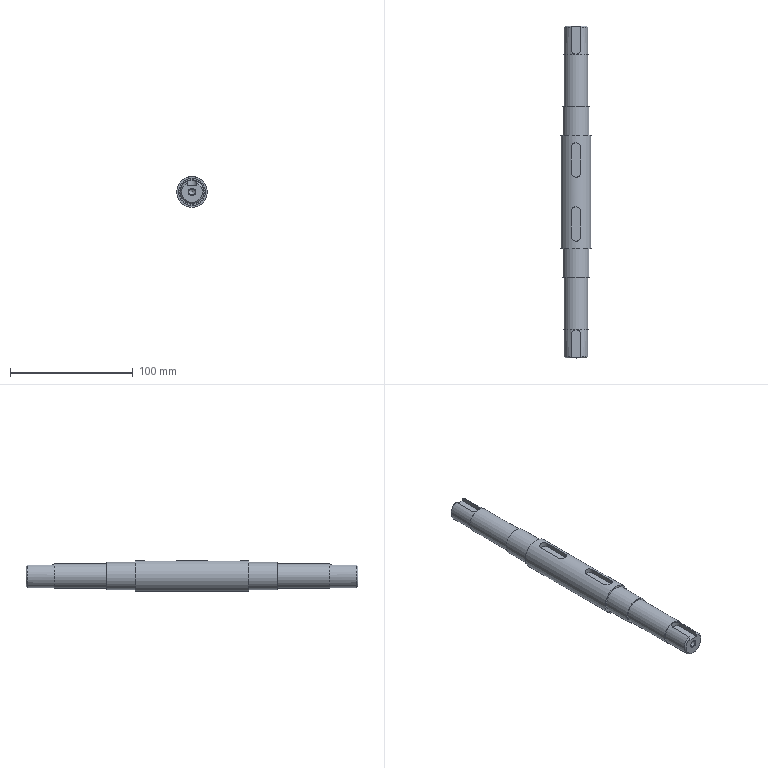Part | STEP file | 冲床-300配套压波_id430_x_t | 1 solid | 41 faces | box 25 x 270 x 25 mm | volume 98996 mm3 | plane 20 | cylinder 15 | cone 6 | commonest cylinder face diameters 8 x6 5 x2 19 x2 20 x2 22 x2 25 x1
STEP:
#1=CARTESIAN_POINT('',(1392.,115.,77.583));
#2=VERTEX_POINT('',#1);
#3=CARTESIAN_POINT('',(1392.,115.,80.083));
#4=DIRECTION('',(0.,1.,0.));
#5=DIRECTION('',(0.,0.,-1.));
#6=AXIS2_PLACEMENT_3D('',#3,#4,#5);
#7=CIRCLE('',#6,2.5);
#8=EDGE_CURVE('',#2,#2,#7,.T.);
#9=ORIENTED_EDGE('',*,*,#8,.T.);
#10=EDGE_LOOP('',(#9));
#11=FACE_BOUND('',#10,.T.);
#12=CARTESIAN_POINT('',(1392.,113.498,80.083));
#13=VERTEX_POINT('',#12);
#14=VERTEX_LOOP('',#13);
#15=FACE_BOUND('',#14,.T.);
#16=CARTESIAN_POINT('',(1392.,115.,80.083));
#17=DIRECTION('',(0.,1.,0.));
#18=DIRECTION('',(0.,0.,1.));
#19=AXIS2_PLACEMENT_3D('',#16,#17,#18);
#20=CONICAL_SURFACE('',#19,2.5,59.);
#21=ADVANCED_FACE('',(#11,#15),#20,.F.);
#22=CARTESIAN_POINT('',(1392.,134.5,77.583));
#23=VERTEX_POINT('',#22);
#24=CARTESIAN_POINT('',(1392.,134.5,80.083));
#25=DIRECTION('',(0.,1.,0.));
#26=DIRECTION('',(0.,0.,-1.));
#27=AXIS2_PLACEMENT_3D('',#24,#25,#26);
#28=CIRCLE('',#27,2.5);
#29=EDGE_CURVE('',#23,#23,#28,.T.);
#30=ORIENTED_EDGE('',*,*,#29,.T.);
#31=EDGE_LOOP('',(#30));
#32=FACE_BOUND('',#31,.T.);
#33=ORIENTED_EDGE('',*,*,#8,.F.);
#34=EDGE_LOOP('',(#33));
#35=FACE_BOUND('',#34,.T.);
#36=CARTESIAN_POINT('',(1392.,135.,80.083));
#37=DIRECTION('',(0.,-1.,0.));
#38=DIRECTION('',(0.,0.,-1.));
#39=AXIS2_PLACEMENT_3D('',#36,#37,#38);
#40=CYLINDRICAL_SURFACE('',#39,2.5);
#41=ADVANCED_FACE('',(#32,#35),#40,.F.);
#42=ORIENTED_EDGE('',*,*,#29,.F.);
#43=EDGE_LOOP('',(#42));
#44=FACE_BOUND('',#43,.T.);
#45=CARTESIAN_POINT('',(1392.,135.,77.083));
#46=VERTEX_POINT('',#45);
#47=CARTESIAN_POINT('',(1392.,135.,80.083));
#48=DIRECTION('',(0.,-1.,0.));
#49=DIRECTION('',(0.,0.,-1.));
#50=AXIS2_PLACEMENT_3D('',#47,#48,#49);
#51=CIRCLE('',#50,3.);
#52=EDGE_CURVE('',#46,#46,#51,.T.);
#53=ORIENTED_EDGE('',*,*,#52,.F.);
#54=EDGE_LOOP('',(#53));
#55=FACE_BOUND('',#54,.T.);
#56=CARTESIAN_POINT('',(1392.,135.,80.083));
#57=DIRECTION('',(0.,1.,0.));
#58=DIRECTION('',(0.,0.,1.));
#59=AXIS2_PLACEMENT_3D('',#56,#57,#58);
#60=CONICAL_SURFACE('',#59,3.,45.);
#61=ADVANCED_FACE('',(#44,#55),#60,.F.);
#62=CARTESIAN_POINT('',(1396.,116.,85.583));
#63=VERTEX_POINT('',#62);
#64=CARTESIAN_POINT('',(1396.,135.,85.583));
#65=VERTEX_POINT('',#64);
#66=CARTESIAN_POINT('',(1396.,114.5,85.583));
#67=DIRECTION('',(0.,1.,0.));
#68=VECTOR('',#67,1.);
#69=LINE('',#66,#68);
#70=EDGE_CURVE('',#63,#65,#69,.T.);
#71=ORIENTED_EDGE('',*,*,#70,.T.);
#72=CARTESIAN_POINT('',(1388.,135.,85.583));
#73=VERTEX_POINT('',#72);
#74=CARTESIAN_POINT('',(1392.,135.,85.583));
#75=DIRECTION('',(1.,0.,0.));
#76=VECTOR('',#75,1.);
#77=LINE('',#74,#76);
#78=EDGE_CURVE('',#73,#65,#77,.T.);
#79=ORIENTED_EDGE('',*,*,#78,.F.);
#80=CARTESIAN_POINT('',(1388.,116.,85.583));
#81=VERTEX_POINT('',#80);
#82=CARTESIAN_POINT('',(1388.,139.499,85.583));
#83=DIRECTION('',(0.,-1.,0.));
#84=VECTOR('',#83,1.);
#85=LINE('',#82,#84);
#86=EDGE_CURVE('',#73,#81,#85,.T.);
#87=ORIENTED_EDGE('',*,*,#86,.T.);
#88=CARTESIAN_POINT('',(1392.,116.,85.583));
#89=DIRECTION('',(0.,0.,1.));
#90=DIRECTION('',(1.,0.,0.));
#91=AXIS2_PLACEMENT_3D('',#88,#89,#90);
#92=CIRCLE('',#91,4.);
#93=EDGE_CURVE('',#81,#63,#92,.T.);
#94=ORIENTED_EDGE('',*,*,#93,.T.);
#95=EDGE_LOOP('',(#71,#79,#87,#94));
#96=FACE_OUTER_BOUND('',#95,.T.);
#97=CARTESIAN_POINT('',(1392.,114.5,85.583));
#98=DIRECTION('',(0.,0.,-1.));
#99=DIRECTION('',(-1.,0.,0.));
#100=AXIS2_PLACEMENT_3D('',#97,#98,#99);
#101=PLANE('',#100);
#102=ADVANCED_FACE('',(#96),#101,.F.);
#103=ORIENTED_EDGE('',*,*,#52,.T.);
#104=EDGE_LOOP('',(#103));
#105=FACE_BOUND('',#104,.T.);
#106=CARTESIAN_POINT('',(1396.,135.,87.583));
#107=VERTEX_POINT('',#106);
#108=CARTESIAN_POINT('',(1396.,135.,80.083));
#109=DIRECTION('',(0.,0.,-1.));
#110=VECTOR('',#109,1.);
#111=LINE('',#108,#110);
#112=EDGE_CURVE('',#107,#65,#111,.T.);
#113=ORIENTED_EDGE('',*,*,#112,.F.);
#114=CARTESIAN_POINT('',(1388.,135.,87.583));
#115=VERTEX_POINT('',#114);
#116=CARTESIAN_POINT('',(1392.,135.,80.083));
#117=DIRECTION('',(0.,1.,0.));
#118=DIRECTION('',(0.,0.,-1.));
#119=AXIS2_PLACEMENT_3D('',#116,#117,#118);
#120=CIRCLE('',#119,8.5);
#121=EDGE_CURVE('',#107,#115,#120,.T.);
#122=ORIENTED_EDGE('',*,*,#121,.T.);
#123=CARTESIAN_POINT('',(1388.,135.,80.083));
#124=DIRECTION('',(0.,0.,1.));
#125=VECTOR('',#124,1.);
#126=LINE('',#123,#125);
#127=EDGE_CURVE('',#73,#115,#126,.T.);
#128=ORIENTED_EDGE('',*,*,#127,.F.);
#129=ORIENTED_EDGE('',*,*,#78,.T.);
#130=EDGE_LOOP('',(#113,#122,#128,#129));
#131=FACE_BOUND('',#130,.T.);
#132=CARTESIAN_POINT('',(1392.,135.,80.083));
#133=DIRECTION('',(0.,-1.,0.));
#134=DIRECTION('',(-1.,0.,0.));
#135=AXIS2_PLACEMENT_3D('',#132,#133,#134);
#136=PLANE('',#135);
#137=ADVANCED_FACE('',(#105,#131),#136,.F.);
#138=CARTESIAN_POINT('',(1388.,116.,88.7));
#139=VERTEX_POINT('',#138);
#140=CARTESIAN_POINT('',(1388.,116.,85.583));
#141=DIRECTION('',(0.,0.,1.));
#142=VECTOR('',#141,1.);
#143=LINE('',#140,#142);
#144=EDGE_CURVE('',#81,#139,#143,.T.);
#145=ORIENTED_EDGE('',*,*,#144,.T.);
#146=CARTESIAN_POINT('',(1392.,112.,89.583));
#147=VERTEX_POINT('',#146);
#148=CARTESIAN_POINT('',(1388.,116.,88.7));
#149=CARTESIAN_POINT('',(1388.,114.929,88.7));
#150=CARTESIAN_POINT('',(1388.443,113.9,88.925));
#151=CARTESIAN_POINT('',(1389.902,112.442,89.38));
#152=CARTESIAN_POINT('',(1390.941,112.,89.583));
#153=CARTESIAN_POINT('',(1392.,112.,89.583));
#154=B_SPLINE_CURVE_WITH_KNOTS('',3,(#148,#149,#150,#151,#152,#153),.UNSPECIFIED.,.F.,.F.,(4,2,4),(0.,0.5,1.),.UNSPECIFIED.);
#155=EDGE_CURVE('',#139,#147,#154,.T.);
#156=ORIENTED_EDGE('',*,*,#155,.T.);
#157=CARTESIAN_POINT('',(1396.,116.,88.7));
#158=VERTEX_POINT('',#157);
#159=CARTESIAN_POINT('',(1392.,112.,89.583));
#160=CARTESIAN_POINT('',(1393.057,112.,89.583));
#161=CARTESIAN_POINT('',(1394.101,112.443,89.38));
#162=CARTESIAN_POINT('',(1395.56,113.904,88.924));
#163=CARTESIAN_POINT('',(1396.,114.93,88.7));
#164=CARTESIAN_POINT('',(1396.,116.,88.7));
#165=B_SPLINE_CURVE_WITH_KNOTS('',3,(#159,#160,#161,#162,#163,#164),.UNSPECIFIED.,.F.,.F.,(4,2,4),(0.,0.5,1.),.UNSPECIFIED.);
#166=EDGE_CURVE('',#147,#158,#165,.T.);
#167=ORIENTED_EDGE('',*,*,#166,.T.);
#168=CARTESIAN_POINT('',(1396.,116.,85.583));
#169=DIRECTION('',(0.,0.,1.));
#170=VECTOR('',#169,1.);
#171=LINE('',#168,#170);
#172=EDGE_CURVE('',#63,#158,#171,.T.);
#173=ORIENTED_EDGE('',*,*,#172,.F.);
#174=ORIENTED_EDGE('',*,*,#93,.F.);
#175=EDGE_LOOP('',(#145,#156,#167,#173,#174));
#176=FACE_OUTER_BOUND('',#175,.T.);
#177=CARTESIAN_POINT('',(1392.,116.,85.583));
#178=DIRECTION('',(0.,0.,1.));
#179=DIRECTION('',(1.,0.,0.));
#180=AXIS2_PLACEMENT_3D('',#177,#178,#179);
#181=CYLINDRICAL_SURFACE('',#180,4.);
#182=ADVANCED_FACE('',(#176),#181,.F.);
#183=CARTESIAN_POINT('',(1396.,134.,88.7));
#184=VERTEX_POINT('',#183);
#185=CARTESIAN_POINT('',(1396.,49.5,88.7));
#186=DIRECTION('',(0.,1.,0.));
#187=VECTOR('',#186,1.);
#188=LINE('',#185,#187);
#189=EDGE_CURVE('',#158,#184,#188,.T.);
#190=ORIENTED_EDGE('',*,*,#189,.T.);
#191=CARTESIAN_POINT('',(1396.,134.,88.7));
#192=CARTESIAN_POINT('',(1396.,134.336,88.33));
#193=CARTESIAN_POINT('',(1396.,134.669,87.958));
#194=CARTESIAN_POINT('',(1396.,135.,87.583));
#195=B_SPLINE_CURVE_WITH_KNOTS('',3,(#191,#192,#193,#194),.UNSPECIFIED.,.F.,.F.,(4,4),(0.,1.),.UNSPECIFIED.);
#196=EDGE_CURVE('',#184,#107,#195,.T.);
#197=ORIENTED_EDGE('',*,*,#196,.T.);
#198=ORIENTED_EDGE('',*,*,#112,.T.);
#199=ORIENTED_EDGE('',*,*,#70,.F.);
#200=ORIENTED_EDGE('',*,*,#172,.T.);
#201=EDGE_LOOP('',(#190,#197,#198,#199,#200));
#202=FACE_OUTER_BOUND('',#201,.T.);
#203=CARTESIAN_POINT('',(1396.,114.5,85.583));
#204=DIRECTION('',(-1.,0.,0.));
#205=DIRECTION('',(0.,1.,0.));
#206=AXIS2_PLACEMENT_3D('',#203,#204,#205);
#207=PLANE('',#206);
#208=ADVANCED_FACE('',(#202),#207,.T.);
#209=CARTESIAN_POINT('',(1388.,134.,88.7));
#210=VERTEX_POINT('',#209);
#211=CARTESIAN_POINT('',(1388.,135.,87.583));
#212=CARTESIAN_POINT('',(1388.,134.669,87.958));
#213=CARTESIAN_POINT('',(1388.,134.336,88.33));
#214=CARTESIAN_POINT('',(1388.,134.,88.7));
#215=B_SPLINE_CURVE_WITH_KNOTS('',3,(#211,#212,#213,#214),.UNSPECIFIED.,.F.,.F.,(4,4),(0.,1.),.UNSPECIFIED.);
#216=EDGE_CURVE('',#115,#210,#215,.T.);
#217=ORIENTED_EDGE('',*,*,#216,.F.);
#218=ORIENTED_EDGE('',*,*,#121,.F.);
#219=ORIENTED_EDGE('',*,*,#196,.F.);
#220=CARTESIAN_POINT('',(1392.,134.,80.083));
#221=DIRECTION('',(0.,-1.,0.));
#222=DIRECTION('',(0.,0.,-1.));
#223=AXIS2_PLACEMENT_3D('',#220,#221,#222);
#224=CIRCLE('',#223,9.5);
#225=EDGE_CURVE('',#210,#184,#224,.T.);
#226=ORIENTED_EDGE('',*,*,#225,.F.);
#227=EDGE_LOOP('',(#217,#218,#219,#226));
#228=FACE_OUTER_BOUND('',#227,.T.);
#229=CARTESIAN_POINT('',(1392.,134.,80.083));
#230=DIRECTION('',(0.,-1.,0.));
#231=DIRECTION('',(0.,0.,-1.));
#232=AXIS2_PLACEMENT_3D('',#229,#230,#231);
#233=CONICAL_SURFACE('',#232,9.5,45.);
#234=ADVANCED_FACE('',(#228),#233,.T.);
#235=ORIENTED_EDGE('',*,*,#127,.T.);
#236=ORIENTED_EDGE('',*,*,#216,.T.);
#237=CARTESIAN_POINT('',(1388.,49.5,88.7));
#238=DIRECTION('',(0.,-1.,0.));
#239=VECTOR('',#238,1.);
#240=LINE('',#237,#239);
#241=EDGE_CURVE('',#210,#139,#240,.T.);
#242=ORIENTED_EDGE('',*,*,#241,.T.);
#243=ORIENTED_EDGE('',*,*,#144,.F.);
#244=ORIENTED_EDGE('',*,*,#86,.F.);
#245=EDGE_LOOP('',(#235,#236,#242,#243,#244));
#246=FACE_OUTER_BOUND('',#245,.T.);
#247=CARTESIAN_POINT('',(1388.,139.499,85.583));
#248=DIRECTION('',(1.,0.,0.));
#249=DIRECTION('',(0.,0.,-1.));
#250=AXIS2_PLACEMENT_3D('',#247,#248,#249);
#251=PLANE('',#250);
#252=ADVANCED_FACE('',(#246),#251,.T.);
#253=ORIENTED_EDGE('',*,*,#241,.F.);
#254=ORIENTED_EDGE('',*,*,#225,.T.);
#255=ORIENTED_EDGE('',*,*,#189,.F.);
#256=ORIENTED_EDGE('',*,*,#166,.F.);
#257=CARTESIAN_POINT('',(1392.,112.,80.083));
#258=DIRECTION('',(0.,-1.,0.));
#259=DIRECTION('',(0.,0.,-1.));
#260=AXIS2_PLACEMENT_3D('',#257,#258,#259);
#261=CIRCLE('',#260,9.5);
#262=EDGE_CURVE('',#147,#147,#261,.T.);
#263=ORIENTED_EDGE('',*,*,#262,.F.);
#264=ORIENTED_EDGE('',*,*,#155,.F.);
#265=EDGE_LOOP('',(#253,#254,#255,#256,#263,#264));
#266=FACE_OUTER_BOUND('',#265,.T.);
#267=CARTESIAN_POINT('',(1392.,49.5,80.083));
#268=DIRECTION('',(0.,1.,0.));
#269=DIRECTION('',(0.,0.,1.));
#270=AXIS2_PLACEMENT_3D('',#267,#268,#269);
#271=CYLINDRICAL_SURFACE('',#270,9.5);
#272=ADVANCED_FACE('',(#266),#271,.T.);
#273=CARTESIAN_POINT('',(1392.,112.,70.083));
#274=VERTEX_POINT('',#273);
#275=CARTESIAN_POINT('',(1392.,112.,80.083));
#276=DIRECTION('',(0.,1.,0.));
#277=DIRECTION('',(0.,0.,-1.));
#278=AXIS2_PLACEMENT_3D('',#275,#276,#277);
#279=CIRCLE('',#278,10.);
#280=EDGE_CURVE('',#274,#274,#279,.T.);
#281=ORIENTED_EDGE('',*,*,#280,.T.);
#282=EDGE_LOOP('',(#281));
#283=FACE_BOUND('',#282,.T.);
#284=ORIENTED_EDGE('',*,*,#262,.T.);
#285=EDGE_LOOP('',(#284));
#286=FACE_BOUND('',#285,.T.);
#287=CARTESIAN_POINT('',(1392.,112.,80.083));
#288=DIRECTION('',(0.,-1.,0.));
#289=DIRECTION('',(-0.2164,0.,-0.9763));
#290=AXIS2_PLACEMENT_3D('',#287,#288,#289);
#291=PLANE('',#290);
#292=ADVANCED_FACE('',(#283,#286),#291,.F.);
#293=ORIENTED_EDGE('',*,*,#280,.F.);
#294=EDGE_LOOP('',(#293));
#295=FACE_BOUND('',#294,.T.);
#296=CARTESIAN_POINT('',(1392.,69.5,70.083));
#297=VERTEX_POINT('',#296);
#298=CARTESIAN_POINT('',(1392.,69.5,80.083));
#299=DIRECTION('',(0.,1.,0.));
#300=DIRECTION('',(0.,0.,-1.));
#301=AXIS2_PLACEMENT_3D('',#298,#299,#300);
#302=CIRCLE('',#301,10.);
#303=EDGE_CURVE('',#297,#297,#302,.T.);
#304=ORIENTED_EDGE('',*,*,#303,.T.);
#305=EDGE_LOOP('',(#304));
#306=FACE_BOUND('',#305,.T.);
#307=CARTESIAN_POINT('',(1392.,679.6,80.083));
#308=DIRECTION('',(0.,-1.,0.));
#309=DIRECTION('',(0.,0.,-1.));
#310=AXIS2_PLACEMENT_3D('',#307,#308,#309);
#311=CYLINDRICAL_SURFACE('',#310,10.);
#312=ADVANCED_FACE('',(#295,#306),#311,.T.);
#313=CARTESIAN_POINT('',(1392.,46.,92.583));
#314=VERTEX_POINT('',#313);
#315=CARTESIAN_POINT('',(1392.,46.,80.083));
#316=DIRECTION('',(0.,1.,0.));
#317=DIRECTION('',(0.,0.,1.));
#318=AXIS2_PLACEMENT_3D('',#315,#316,#317);
#319=CIRCLE('',#318,12.5);
#320=EDGE_CURVE('',#314,#314,#319,.T.);
#321=ORIENTED_EDGE('',*,*,#320,.F.);
#322=EDGE_LOOP('',(#321));
#323=FACE_BOUND('',#322,.T.);
#324=CARTESIAN_POINT('',(1396.,36.,91.926));
#325=VERTEX_POINT('',#324);
#326=CARTESIAN_POINT('',(1388.,36.,91.926));
#327=VERTEX_POINT('',#326);
#328=CARTESIAN_POINT('',(1396.,36.,91.926));
#329=CARTESIAN_POINT('',(1396.,36.205,91.926));
#330=CARTESIAN_POINT('',(1395.984,36.412,91.932));
#331=CARTESIAN_POINT('',(1395.953,36.614,91.942));
#332=CARTESIAN_POINT('',(1395.882,37.066,91.966));
#333=CARTESIAN_POINT('',(1395.731,37.51,92.016));
#334=CARTESIAN_POINT('',(1395.515,37.909,92.079));
#335=CARTESIAN_POINT('',(1395.301,38.303,92.142));
#336=CARTESIAN_POINT('',(1395.018,38.663,92.218));
#337=CARTESIAN_POINT('',(1394.687,38.963,92.291));
#338=CARTESIAN_POINT('',(1394.37,39.251,92.361));
#339=CARTESIAN_POINT('',(1394.001,39.49,92.429));
#340=CARTESIAN_POINT('',(1393.607,39.663,92.48));
#341=CARTESIAN_POINT('',(1393.218,39.834,92.53));
#342=CARTESIAN_POINT('',(1392.793,39.944,92.566));
#343=CARTESIAN_POINT('',(1392.367,39.983,92.578));
#344=CARTESIAN_POINT('',(1391.925,40.024,92.591));
#345=CARTESIAN_POINT('',(1391.469,39.989,92.58));
#346=CARTESIAN_POINT('',(1391.039,39.883,92.547));
#347=CARTESIAN_POINT('',(1390.595,39.773,92.512));
#348=CARTESIAN_POINT('',(1390.166,39.583,92.454));
#349=CARTESIAN_POINT('',(1389.788,39.332,92.386));
#350=CARTESIAN_POINT('',(1389.418,39.087,92.32));
#351=CARTESIAN_POINT('',(1389.087,38.777,92.242));
#352=CARTESIAN_POINT('',(1388.818,38.424,92.172));
#353=CARTESIAN_POINT('',(1388.559,38.083,92.103));
#354=CARTESIAN_POINT('',(1388.351,37.694,92.04));
#355=CARTESIAN_POINT('',(1388.212,37.285,91.996));
#356=CARTESIAN_POINT('',(1388.073,36.875,91.952));
#357=CARTESIAN_POINT('',(1388.,36.435,91.926));
#358=CARTESIAN_POINT('',(1388.,36.,91.926));
#359=B_SPLINE_CURVE_WITH_KNOTS('',3,(#328,#329,#330,#331,#332,#333,#334,#335,#336,#337,#338,#339,#340,#341,#342,#343,#344,#345,#346,#347,#348,#349,#350,#351,#352,#353,#354,#355,#356,#357,#358),.UNSPECIFIED.,.F.,.F.,(4,3,3,3,3,3,3,3,3,3,4),(0.,0.04841,0.1576,0.2655,0.3687,0.4707,0.5766,0.6861,0.7929,0.8964,1.),.UNSPECIFIED.);
#360=EDGE_CURVE('',#325,#327,#359,.T.);
#361=ORIENTED_EDGE('',*,*,#360,.F.);
#362=CARTESIAN_POINT('',(1396.,16.,91.926));
#363=VERTEX_POINT('',#362);
#364=CARTESIAN_POINT('',(1396.,-46.,91.926));
#365=DIRECTION('',(0.,1.,0.));
#366=VECTOR('',#365,1.);
#367=LINE('',#364,#366);
#368=EDGE_CURVE('',#363,#325,#367,.T.);
#369=ORIENTED_EDGE('',*,*,#368,.F.);
#370=CARTESIAN_POINT('',(1388.,16.,91.926));
#371=VERTEX_POINT('',#370);
#372=CARTESIAN_POINT('',(1388.,16.,91.926));
#373=CARTESIAN_POINT('',(1388.,15.565,91.926));
#374=CARTESIAN_POINT('',(1388.073,15.125,91.952));
#375=CARTESIAN_POINT('',(1388.212,14.715,91.996));
#376=CARTESIAN_POINT('',(1388.351,14.306,92.04));
#377=CARTESIAN_POINT('',(1388.559,13.917,92.103));
#378=CARTESIAN_POINT('',(1388.818,13.576,92.172));
#379=CARTESIAN_POINT('',(1389.087,13.223,92.242));
#380=CARTESIAN_POINT('',(1389.418,12.913,92.32));
#381=CARTESIAN_POINT('',(1389.788,12.668,92.386));
#382=CARTESIAN_POINT('',(1390.166,12.417,92.454));
#383=CARTESIAN_POINT('',(1390.595,12.227,92.512));
#384=CARTESIAN_POINT('',(1391.039,12.117,92.547));
#385=CARTESIAN_POINT('',(1391.469,12.011,92.58));
#386=CARTESIAN_POINT('',(1391.925,11.976,92.591));
#387=CARTESIAN_POINT('',(1392.367,12.017,92.578));
#388=CARTESIAN_POINT('',(1392.793,12.056,92.566));
#389=CARTESIAN_POINT('',(1393.218,12.166,92.53));
#390=CARTESIAN_POINT('',(1393.607,12.337,92.48));
#391=CARTESIAN_POINT('',(1394.001,12.51,92.429));
#392=CARTESIAN_POINT('',(1394.37,12.749,92.361));
#393=CARTESIAN_POINT('',(1394.687,13.037,92.291));
#394=CARTESIAN_POINT('',(1395.018,13.337,92.218));
#395=CARTESIAN_POINT('',(1395.301,13.697,92.142));
#396=CARTESIAN_POINT('',(1395.515,14.091,92.079));
#397=CARTESIAN_POINT('',(1395.731,14.49,92.016));
#398=CARTESIAN_POINT('',(1395.882,14.934,91.966));
#399=CARTESIAN_POINT('',(1395.953,15.386,91.942));
#400=CARTESIAN_POINT('',(1395.984,15.588,91.932));
#401=CARTESIAN_POINT('',(1396.,15.795,91.926));
#402=CARTESIAN_POINT('',(1396.,16.,91.926));
#403=B_SPLINE_CURVE_WITH_KNOTS('',3,(#372,#373,#374,#375,#376,#377,#378,#379,#380,#381,#382,#383,#384,#385,#386,#387,#388,#389,#390,#391,#392,#393,#394,#395,#396,#397,#398,#399,#400,#401,#402),.UNSPECIFIED.,.F.,.F.,(4,3,3,3,3,3,3,3,3,3,4),(0.,0.1036,0.2071,0.3139,0.4234,0.5293,0.6313,0.7345,0.8424,0.9516,1.),.UNSPECIFIED.);
#404=EDGE_CURVE('',#371,#363,#403,.T.);
#405=ORIENTED_EDGE('',*,*,#404,.F.);
#406=CARTESIAN_POINT('',(1388.,-46.,91.926));
#407=DIRECTION('',(0.,-1.,0.));
#408=VECTOR('',#407,1.);
#409=LINE('',#406,#408);
#410=EDGE_CURVE('',#327,#371,#409,.T.);
#411=ORIENTED_EDGE('',*,*,#410,.F.);
#412=EDGE_LOOP('',(#361,#369,#405,#411));
#413=FACE_BOUND('',#412,.T.);
#414=CARTESIAN_POINT('',(1392.,-46.,92.583));
#415=VERTEX_POINT('',#414);
#416=CARTESIAN_POINT('',(1392.,-46.,80.083));
#417=DIRECTION('',(0.,-1.,0.));
#418=DIRECTION('',(0.,0.,1.));
#419=AXIS2_PLACEMENT_3D('',#416,#417,#418);
#420=CIRCLE('',#419,12.5);
#421=EDGE_CURVE('',#415,#415,#420,.T.);
#422=ORIENTED_EDGE('',*,*,#421,.F.);
#423=EDGE_LOOP('',(#422));
#424=FACE_BOUND('',#423,.T.);
#425=CARTESIAN_POINT('',(1388.,-36.,91.926));
#426=VERTEX_POINT('',#425);
#427=CARTESIAN_POINT('',(1396.,-36.,91.926));
#428=VERTEX_POINT('',#427);
#429=CARTESIAN_POINT('',(1388.,-36.,91.926));
#430=CARTESIAN_POINT('',(1388.,-36.435,91.926));
#431=CARTESIAN_POINT('',(1388.073,-36.875,91.952));
#432=CARTESIAN_POINT('',(1388.212,-37.285,91.996));
#433=CARTESIAN_POINT('',(1388.351,-37.694,92.04));
#434=CARTESIAN_POINT('',(1388.559,-38.083,92.103));
#435=CARTESIAN_POINT('',(1388.818,-38.424,92.172));
#436=CARTESIAN_POINT('',(1389.087,-38.777,92.242));
#437=CARTESIAN_POINT('',(1389.418,-39.087,92.32));
#438=CARTESIAN_POINT('',(1389.788,-39.332,92.386));
#439=CARTESIAN_POINT('',(1390.166,-39.583,92.454));
#440=CARTESIAN_POINT('',(1390.595,-39.773,92.512));
#441=CARTESIAN_POINT('',(1391.039,-39.883,92.547));
#442=CARTESIAN_POINT('',(1391.469,-39.989,92.58));
#443=CARTESIAN_POINT('',(1391.925,-40.024,92.591));
#444=CARTESIAN_POINT('',(1392.367,-39.983,92.578));
#445=CARTESIAN_POINT('',(1392.793,-39.944,92.566));
#446=CARTESIAN_POINT('',(1393.218,-39.834,92.53));
#447=CARTESIAN_POINT('',(1393.607,-39.663,92.48));
#448=CARTESIAN_POINT('',(1394.001,-39.49,92.429));
#449=CARTESIAN_POINT('',(1394.37,-39.251,92.361));
#450=CARTESIAN_POINT('',(1394.687,-38.963,92.291));
#451=CARTESIAN_POINT('',(1395.018,-38.663,92.218));
#452=CARTESIAN_POINT('',(1395.301,-38.303,92.142));
#453=CARTESIAN_POINT('',(1395.515,-37.909,92.079));
#454=CARTESIAN_POINT('',(1395.731,-37.51,92.016));
#455=CARTESIAN_POINT('',(1395.882,-37.066,91.966));
#456=CARTESIAN_POINT('',(1395.953,-36.614,91.942));
#457=CARTESIAN_POINT('',(1395.984,-36.412,91.932));
#458=CARTESIAN_POINT('',(1396.,-36.205,91.926));
#459=CARTESIAN_POINT('',(1396.,-36.,91.926));
#460=B_SPLINE_CURVE_WITH_KNOTS('',3,(#429,#430,#431,#432,#433,#434,#435,#436,#437,#438,#439,#440,#441,#442,#443,#444,#445,#446,#447,#448,#449,#450,#451,#452,#453,#454,#455,#456,#457,#458,#459),.UNSPECIFIED.,.F.,.F.,(4,3,3,3,3,3,3,3,3,3,4),(0.,0.1036,0.2071,0.3139,0.4234,0.5293,0.6313,0.7345,0.8424,0.9516,1.),.UNSPECIFIED.);
#461=EDGE_CURVE('',#426,#428,#460,.T.);
#462=ORIENTED_EDGE('',*,*,#461,.F.);
#463=CARTESIAN_POINT('',(1388.,-16.,91.926));
#464=VERTEX_POINT('',#463);
#465=CARTESIAN_POINT('',(1388.,46.,91.926));
#466=DIRECTION('',(0.,-1.,0.));
#467=VECTOR('',#466,1.);
#468=LINE('',#465,#467);
#469=EDGE_CURVE('',#464,#426,#468,.T.);
#470=ORIENTED_EDGE('',*,*,#469,.F.);
#471=CARTESIAN_POINT('',(1396.,-16.,91.926));
#472=VERTEX_POINT('',#471);
#473=CARTESIAN_POINT('',(1396.,-16.,91.926));
#474=CARTESIAN_POINT('',(1396.,-15.565,91.926));
#475=CARTESIAN_POINT('',(1395.927,-15.125,91.952));
#476=CARTESIAN_POINT('',(1395.788,-14.715,91.996));
#477=CARTESIAN_POINT('',(1395.649,-14.306,92.04));
#478=CARTESIAN_POINT('',(1395.441,-13.917,92.103));
#479=CARTESIAN_POINT('',(1395.182,-13.576,92.172));
#480=CARTESIAN_POINT('',(1394.913,-13.223,92.242));
#481=CARTESIAN_POINT('',(1394.582,-12.913,92.32));
#482=CARTESIAN_POINT('',(1394.212,-12.668,92.386));
#483=CARTESIAN_POINT('',(1393.834,-12.417,92.454));
#484=CARTESIAN_POINT('',(1393.405,-12.227,92.512));
#485=CARTESIAN_POINT('',(1392.961,-12.117,92.547));
#486=CARTESIAN_POINT('',(1392.531,-12.011,92.58));
#487=CARTESIAN_POINT('',(1392.075,-11.976,92.591));
#488=CARTESIAN_POINT('',(1391.633,-12.017,92.578));
#489=CARTESIAN_POINT('',(1391.207,-12.056,92.566));
#490=CARTESIAN_POINT('',(1390.782,-12.166,92.53));
#491=CARTESIAN_POINT('',(1390.393,-12.337,92.48));
#492=CARTESIAN_POINT('',(1389.999,-12.51,92.429));
#493=CARTESIAN_POINT('',(1389.63,-12.749,92.361));
#494=CARTESIAN_POINT('',(1389.313,-13.037,92.291));
#495=CARTESIAN_POINT('',(1388.982,-13.337,92.218));
#496=CARTESIAN_POINT('',(1388.699,-13.697,92.142));
#497=CARTESIAN_POINT('',(1388.485,-14.091,92.079));
#498=CARTESIAN_POINT('',(1388.269,-14.49,92.016));
#499=CARTESIAN_POINT('',(1388.118,-14.934,91.966));
#500=CARTESIAN_POINT('',(1388.047,-15.386,91.942));
#501=CARTESIAN_POINT('',(1388.016,-15.588,91.932));
#502=CARTESIAN_POINT('',(1388.,-15.795,91.926));
#503=CARTESIAN_POINT('',(1388.,-16.,91.926));
#504=B_SPLINE_CURVE_WITH_KNOTS('',3,(#473,#474,#475,#476,#477,#478,#479,#480,#481,#482,#483,#484,#485,#486,#487,#488,#489,#490,#491,#492,#493,#494,#495,#496,#497,#498,#499,#500,#501,#502,#503),.UNSPECIFIED.,.F.,.F.,(4,3,3,3,3,3,3,3,3,3,4),(0.,0.1036,0.2071,0.3139,0.4234,0.5293,0.6313,0.7345,0.8424,0.9516,1.),.UNSPECIFIED.);
#505=EDGE_CURVE('',#472,#464,#504,.T.);
#506=ORIENTED_EDGE('',*,*,#505,.F.);
#507=CARTESIAN_POINT('',(1396.,46.,91.926));
#508=DIRECTION('',(0.,1.,0.));
#509=VECTOR('',#508,1.);
#510=LINE('',#507,#509);
#511=EDGE_CURVE('',#428,#472,#510,.T.);
#512=ORIENTED_EDGE('',*,*,#511,.F.);
#513=EDGE_LOOP('',(#462,#470,#506,#512));
#514=FACE_BOUND('',#513,.T.);
#515=CARTESIAN_POINT('',(1392.,-46.,80.083));
#516=DIRECTION('',(0.,1.,0.));
#517=DIRECTION('',(0.,0.,-1.));
#518=AXIS2_PLACEMENT_3D('',#515,#516,#517);
#519=CYLINDRICAL_SURFACE('',#518,12.5);
#520=ADVANCED_FACE('',(#323,#413,#424,#514),#519,.T.);
#521=CARTESIAN_POINT('',(1392.,69.5,69.083));
#522=VERTEX_POINT('',#521);
#523=CARTESIAN_POINT('',(1392.,69.5,80.083));
#524=DIRECTION('',(0.,-1.,0.));
#525=DIRECTION('',(0.,0.,-1.));
#526=AXIS2_PLACEMENT_3D('',#523,#524,#525);
#527=CIRCLE('',#526,11.);
#528=EDGE_CURVE('',#522,#522,#527,.T.);
#529=ORIENTED_EDGE('',*,*,#528,.T.);
#530=EDGE_LOOP('',(#529));
#531=FACE_BOUND('',#530,.T.);
#532=CARTESIAN_POINT('',(1392.,46.,91.083));
#533=VERTEX_POINT('',#532);
#534=CARTESIAN_POINT('',(1392.,46.,80.083));
#535=DIRECTION('',(0.,-1.,0.));
#536=DIRECTION('',(0.,0.,1.));
#537=AXIS2_PLACEMENT_3D('',#534,#535,#536);
#538=CIRCLE('',#537,11.);
#539=EDGE_CURVE('',#533,#533,#538,.T.);
#540=ORIENTED_EDGE('',*,*,#539,.F.);
#541=EDGE_LOOP('',(#540));
#542=FACE_BOUND('',#541,.T.);
#543=CARTESIAN_POINT('',(1392.,679.6,80.083));
#544=DIRECTION('',(0.,-1.,0.));
#545=DIRECTION('',(0.,0.,-1.));
#546=AXIS2_PLACEMENT_3D('',#543,#544,#545);
#547=CYLINDRICAL_SURFACE('',#546,11.);
#548=ADVANCED_FACE('',(#531,#542),#547,.T.);
#549=ORIENTED_EDGE('',*,*,#539,.T.);
#550=EDGE_LOOP('',(#549));
#551=FACE_BOUND('',#550,.T.);
#552=ORIENTED_EDGE('',*,*,#320,.T.);
#553=EDGE_LOOP('',(#552));
#554=FACE_BOUND('',#553,.T.);
#555=CARTESIAN_POINT('',(1392.,46.,80.083));
#556=DIRECTION('',(0.,1.,0.));
#557=DIRECTION('',(0.,0.,1.));
#558=AXIS2_PLACEMENT_3D('',#555,#556,#557);
#559=PLANE('',#558);
#560=ADVANCED_FACE('',(#551,#554),#559,.T.);
#561=ORIENTED_EDGE('',*,*,#360,.T.);
#562=CARTESIAN_POINT('',(1388.,36.,88.583));
#563=VERTEX_POINT('',#562);
#564=CARTESIAN_POINT('',(1388.,36.,88.583));
#565=DIRECTION('',(0.,0.,1.));
#566=VECTOR('',#565,1.);
#567=LINE('',#564,#566);
#568=EDGE_CURVE('',#563,#327,#567,.T.);
#569=ORIENTED_EDGE('',*,*,#568,.F.);
#570=CARTESIAN_POINT('',(1396.,36.,88.583));
#571=VERTEX_POINT('',#570);
#572=CARTESIAN_POINT('',(1392.,36.,88.583));
#573=DIRECTION('',(0.,0.,-1.));
#574=DIRECTION('',(0.,-1.,0.));
#575=AXIS2_PLACEMENT_3D('',#572,#573,#574);
#576=CIRCLE('',#575,4.);
#577=EDGE_CURVE('',#563,#571,#576,.T.);
#578=ORIENTED_EDGE('',*,*,#577,.T.);
#579=CARTESIAN_POINT('',(1396.,36.,88.583));
#580=DIRECTION('',(0.,0.,1.));
#581=VECTOR('',#580,1.);
#582=LINE('',#579,#581);
#583=EDGE_CURVE('',#571,#325,#582,.T.);
#584=ORIENTED_EDGE('',*,*,#583,.T.);
#585=EDGE_LOOP('',(#561,#569,#578,#584));
#586=FACE_OUTER_BOUND('',#585,.T.);
#587=CARTESIAN_POINT('',(1392.,36.,88.583));
#588=DIRECTION('',(0.,0.,1.));
#589=DIRECTION('',(1.,0.,0.));
#590=AXIS2_PLACEMENT_3D('',#587,#588,#589);
#591=CYLINDRICAL_SURFACE('',#590,4.);
#592=ADVANCED_FACE('',(#586),#591,.F.);
#593=ORIENTED_EDGE('',*,*,#368,.T.);
#594=ORIENTED_EDGE('',*,*,#583,.F.);
#595=CARTESIAN_POINT('',(1396.,16.,88.583));
#596=VERTEX_POINT('',#595);
#597=CARTESIAN_POINT('',(1396.,36.,88.583));
#598=DIRECTION('',(0.,-1.,0.));
#599=VECTOR('',#598,1.);
#600=LINE('',#597,#599);
#601=EDGE_CURVE('',#571,#596,#600,.T.);
#602=ORIENTED_EDGE('',*,*,#601,.T.);
#603=CARTESIAN_POINT('',(1396.,16.,88.583));
#604=DIRECTION('',(0.,0.,1.));
#605=VECTOR('',#604,1.);
#606=LINE('',#603,#605);
#607=EDGE_CURVE('',#596,#363,#606,.T.);
#608=ORIENTED_EDGE('',*,*,#607,.T.);
#609=EDGE_LOOP('',(#593,#594,#602,#608));
#610=FACE_OUTER_BOUND('',#609,.T.);
#611=CARTESIAN_POINT('',(1396.,36.,88.583));
#612=DIRECTION('',(1.,0.,0.));
#613=DIRECTION('',(0.,0.,-1.));
#614=AXIS2_PLACEMENT_3D('',#611,#612,#613);
#615=PLANE('',#614);
#616=ADVANCED_FACE('',(#610),#615,.F.);
#617=ORIENTED_EDGE('',*,*,#404,.T.);
#618=ORIENTED_EDGE('',*,*,#607,.F.);
#619=CARTESIAN_POINT('',(1388.,16.,88.583));
#620=VERTEX_POINT('',#619);
#621=CARTESIAN_POINT('',(1392.,16.,88.583));
#622=DIRECTION('',(0.,0.,-1.));
#623=DIRECTION('',(0.,-1.,0.));
#624=AXIS2_PLACEMENT_3D('',#621,#622,#623);
#625=CIRCLE('',#624,4.);
#626=EDGE_CURVE('',#596,#620,#625,.T.);
#627=ORIENTED_EDGE('',*,*,#626,.T.);
#628=CARTESIAN_POINT('',(1388.,16.,88.583));
#629=DIRECTION('',(0.,0.,1.));
#630=VECTOR('',#629,1.);
#631=LINE('',#628,#630);
#632=EDGE_CURVE('',#620,#371,#631,.T.);
#633=ORIENTED_EDGE('',*,*,#632,.T.);
#634=EDGE_LOOP('',(#617,#618,#627,#633));
#635=FACE_OUTER_BOUND('',#634,.T.);
#636=CARTESIAN_POINT('',(1392.,16.,88.583));
#637=DIRECTION('',(0.,0.,1.));
#638=DIRECTION('',(1.,0.,0.));
#639=AXIS2_PLACEMENT_3D('',#636,#637,#638);
#640=CYLINDRICAL_SURFACE('',#639,4.);
#641=ADVANCED_FACE('',(#635),#640,.F.);
#642=ORIENTED_EDGE('',*,*,#410,.T.);
#643=ORIENTED_EDGE('',*,*,#632,.F.);
#644=CARTESIAN_POINT('',(1388.,16.,88.583));
#645=DIRECTION('',(0.,1.,0.));
#646=VECTOR('',#645,1.);
#647=LINE('',#644,#646);
#648=EDGE_CURVE('',#620,#563,#647,.T.);
#649=ORIENTED_EDGE('',*,*,#648,.T.);
#650=ORIENTED_EDGE('',*,*,#568,.T.);
#651=EDGE_LOOP('',(#642,#643,#649,#650));
#652=FACE_OUTER_BOUND('',#651,.T.);
#653=CARTESIAN_POINT('',(1388.,16.,88.583));
#654=DIRECTION('',(-1.,0.,0.));
#655=DIRECTION('',(0.,0.,1.));
#656=AXIS2_PLACEMENT_3D('',#653,#654,#655);
#657=PLANE('',#656);
#658=ADVANCED_FACE('',(#652),#657,.F.);
#659=ORIENTED_EDGE('',*,*,#577,.F.);
#660=ORIENTED_EDGE('',*,*,#648,.F.);
#661=ORIENTED_EDGE('',*,*,#626,.F.);
#662=ORIENTED_EDGE('',*,*,#601,.F.);
#663=EDGE_LOOP('',(#659,#660,#661,#662));
#664=FACE_OUTER_BOUND('',#663,.T.);
#665=CARTESIAN_POINT('',(1392.,36.,88.583));
#666=DIRECTION('',(0.,0.,1.));
#667=DIRECTION('',(1.,0.,0.));
#668=AXIS2_PLACEMENT_3D('',#665,#666,#667);
#669=PLANE('',#668);
#670=ADVANCED_FACE('',(#664),#669,.T.);
#671=CARTESIAN_POINT('',(1392.,-69.5,91.083));
#672=VERTEX_POINT('',#671);
#673=CARTESIAN_POINT('',(1392.,-69.5,80.083));
#674=DIRECTION('',(0.,1.,0.));
#675=DIRECTION('',(0.,0.,1.));
#676=AXIS2_PLACEMENT_3D('',#673,#674,#675);
#677=CIRCLE('',#676,11.);
#678=EDGE_CURVE('',#672,#672,#677,.T.);
#679=ORIENTED_EDGE('',*,*,#678,.T.);
#680=EDGE_LOOP('',(#679));
#681=FACE_BOUND('',#680,.T.);
#682=CARTESIAN_POINT('',(1392.,-46.,91.083));
#683=VERTEX_POINT('',#682);
#684=CARTESIAN_POINT('',(1392.,-46.,80.083));
#685=DIRECTION('',(0.,1.,0.));
#686=DIRECTION('',(0.,0.,1.));
#687=AXIS2_PLACEMENT_3D('',#684,#685,#686);
#688=CIRCLE('',#687,11.);
#689=EDGE_CURVE('',#683,#683,#688,.T.);
#690=ORIENTED_EDGE('',*,*,#689,.F.);
#691=EDGE_LOOP('',(#690));
#692=FACE_BOUND('',#691,.T.);
#693=CARTESIAN_POINT('',(1392.,-679.6,80.083));
#694=DIRECTION('',(0.,1.,0.));
#695=DIRECTION('',(0.,0.,-1.));
#696=AXIS2_PLACEMENT_3D('',#693,#694,#695);
#697=CYLINDRICAL_SURFACE('',#696,11.);
#698=ADVANCED_FACE('',(#681,#692),#697,.T.);
#699=ORIENTED_EDGE('',*,*,#689,.T.);
#700=EDGE_LOOP('',(#699));
#701=FACE_BOUND('',#700,.T.);
#702=ORIENTED_EDGE('',*,*,#421,.T.);
#703=EDGE_LOOP('',(#702));
#704=FACE_BOUND('',#703,.T.);
#705=CARTESIAN_POINT('',(1392.,-46.,80.083));
#706=DIRECTION('',(0.,-1.,0.));
#707=DIRECTION('',(0.,0.,1.));
#708=AXIS2_PLACEMENT_3D('',#705,#706,#707);
#709=PLANE('',#708);
#710=ADVANCED_FACE('',(#701,#704),#709,.T.);
#711=ORIENTED_EDGE('',*,*,#461,.T.);
#712=CARTESIAN_POINT('',(1396.,-36.,88.583));
#713=VERTEX_POINT('',#712);
#714=CARTESIAN_POINT('',(1396.,-36.,88.583));
#715=DIRECTION('',(0.,0.,-1.));
#716=VECTOR('',#715,1.);
#717=LINE('',#714,#716);
#718=EDGE_CURVE('',#428,#713,#717,.T.);
#719=ORIENTED_EDGE('',*,*,#718,.T.);
#720=CARTESIAN_POINT('',(1388.,-36.,88.583));
#721=VERTEX_POINT('',#720);
#722=CARTESIAN_POINT('',(1392.,-36.,88.583));
#723=DIRECTION('',(0.,0.,-1.));
#724=DIRECTION('',(0.,1.,0.));
#725=AXIS2_PLACEMENT_3D('',#722,#723,#724);
#726=CIRCLE('',#725,4.);
#727=EDGE_CURVE('',#713,#721,#726,.T.);
#728=ORIENTED_EDGE('',*,*,#727,.T.);
#729=CARTESIAN_POINT('',(1388.,-36.,88.583));
#730=DIRECTION('',(0.,0.,-1.));
#731=VECTOR('',#730,1.);
#732=LINE('',#729,#731);
#733=EDGE_CURVE('',#426,#721,#732,.T.);
#734=ORIENTED_EDGE('',*,*,#733,.F.);
#735=EDGE_LOOP('',(#711,#719,#728,#734));
#736=FACE_OUTER_BOUND('',#735,.T.);
#737=CARTESIAN_POINT('',(1392.,-36.,88.583));
#738=DIRECTION('',(0.,0.,1.));
#739=DIRECTION('',(1.,0.,0.));
#740=AXIS2_PLACEMENT_3D('',#737,#738,#739);
#741=CYLINDRICAL_SURFACE('',#740,4.);
#742=ADVANCED_FACE('',(#736),#741,.F.);
#743=ORIENTED_EDGE('',*,*,#511,.T.);
#744=CARTESIAN_POINT('',(1396.,-16.,88.583));
#745=VERTEX_POINT('',#744);
#746=CARTESIAN_POINT('',(1396.,-16.,88.583));
#747=DIRECTION('',(0.,0.,-1.));
#748=VECTOR('',#747,1.);
#749=LINE('',#746,#748);
#750=EDGE_CURVE('',#472,#745,#749,.T.);
#751=ORIENTED_EDGE('',*,*,#750,.T.);
#752=CARTESIAN_POINT('',(1396.,-36.,88.583));
#753=DIRECTION('',(0.,-1.,0.));
#754=VECTOR('',#753,1.);
#755=LINE('',#752,#754);
#756=EDGE_CURVE('',#745,#713,#755,.T.);
#757=ORIENTED_EDGE('',*,*,#756,.T.);
#758=ORIENTED_EDGE('',*,*,#718,.F.);
#759=EDGE_LOOP('',(#743,#751,#757,#758));
#760=FACE_OUTER_BOUND('',#759,.T.);
#761=CARTESIAN_POINT('',(1396.,-36.,88.583));
#762=DIRECTION('',(1.,0.,0.));
#763=DIRECTION('',(0.,0.,-1.));
#764=AXIS2_PLACEMENT_3D('',#761,#762,#763);
#765=PLANE('',#764);
#766=ADVANCED_FACE('',(#760),#765,.F.);
#767=ORIENTED_EDGE('',*,*,#505,.T.);
#768=CARTESIAN_POINT('',(1388.,-16.,88.583));
#769=VERTEX_POINT('',#768);
#770=CARTESIAN_POINT('',(1388.,-16.,88.583));
#771=DIRECTION('',(0.,0.,-1.));
#772=VECTOR('',#771,1.);
#773=LINE('',#770,#772);
#774=EDGE_CURVE('',#464,#769,#773,.T.);
#775=ORIENTED_EDGE('',*,*,#774,.T.);
#776=CARTESIAN_POINT('',(1392.,-16.,88.583));
#777=DIRECTION('',(0.,0.,-1.));
#778=DIRECTION('',(0.,1.,0.));
#779=AXIS2_PLACEMENT_3D('',#776,#777,#778);
#780=CIRCLE('',#779,4.);
#781=EDGE_CURVE('',#769,#745,#780,.T.);
#782=ORIENTED_EDGE('',*,*,#781,.T.);
#783=ORIENTED_EDGE('',*,*,#750,.F.);
#784=EDGE_LOOP('',(#767,#775,#782,#783));
#785=FACE_OUTER_BOUND('',#784,.T.);
#786=CARTESIAN_POINT('',(1392.,-16.,88.583));
#787=DIRECTION('',(0.,0.,1.));
#788=DIRECTION('',(1.,0.,0.));
#789=AXIS2_PLACEMENT_3D('',#786,#787,#788);
#790=CYLINDRICAL_SURFACE('',#789,4.);
#791=ADVANCED_FACE('',(#785),#790,.F.);
#792=ORIENTED_EDGE('',*,*,#469,.T.);
#793=ORIENTED_EDGE('',*,*,#733,.T.);
#794=CARTESIAN_POINT('',(1388.,-16.,88.583));
#795=DIRECTION('',(0.,1.,0.));
#796=VECTOR('',#795,1.);
#797=LINE('',#794,#796);
#798=EDGE_CURVE('',#721,#769,#797,.T.);
#799=ORIENTED_EDGE('',*,*,#798,.T.);
#800=ORIENTED_EDGE('',*,*,#774,.F.);
#801=EDGE_LOOP('',(#792,#793,#799,#800));
#802=FACE_OUTER_BOUND('',#801,.T.);
#803=CARTESIAN_POINT('',(1388.,-16.,88.583));
#804=DIRECTION('',(-1.,0.,0.));
#805=DIRECTION('',(0.,0.,1.));
#806=AXIS2_PLACEMENT_3D('',#803,#804,#805);
#807=PLANE('',#806);
#808=ADVANCED_FACE('',(#802),#807,.F.);
#809=ORIENTED_EDGE('',*,*,#727,.F.);
#810=ORIENTED_EDGE('',*,*,#756,.F.);
#811=ORIENTED_EDGE('',*,*,#781,.F.);
#812=ORIENTED_EDGE('',*,*,#798,.F.);
#813=EDGE_LOOP('',(#809,#810,#811,#812));
#814=FACE_OUTER_BOUND('',#813,.T.);
#815=CARTESIAN_POINT('',(1392.,-36.,88.583));
#816=DIRECTION('',(0.,0.,1.));
#817=DIRECTION('',(1.,0.,0.));
#818=AXIS2_PLACEMENT_3D('',#815,#816,#817);
#819=PLANE('',#818);
#820=ADVANCED_FACE('',(#814),#819,.T.);
#821=CARTESIAN_POINT('',(1392.,-69.5,90.083));
#822=VERTEX_POINT('',#821);
#823=CARTESIAN_POINT('',(1392.,-69.5,80.083));
#824=DIRECTION('',(0.,-1.,0.));
#825=DIRECTION('',(0.,0.,1.));
#826=AXIS2_PLACEMENT_3D('',#823,#824,#825);
#827=CIRCLE('',#826,10.);
#828=EDGE_CURVE('',#822,#822,#827,.T.);
#829=ORIENTED_EDGE('',*,*,#828,.F.);
#830=EDGE_LOOP('',(#829));
#831=FACE_BOUND('',#830,.T.);
#832=ORIENTED_EDGE('',*,*,#678,.F.);
#833=EDGE_LOOP('',(#832));
#834=FACE_BOUND('',#833,.T.);
#835=CARTESIAN_POINT('',(1392.,-69.5,80.083));
#836=DIRECTION('',(0.,1.,0.));
#837=DIRECTION('',(0.,0.,1.));
#838=AXIS2_PLACEMENT_3D('',#835,#836,#837);
#839=PLANE('',#838);
#840=ADVANCED_FACE('',(#831,#834),#839,.F.);
#841=ORIENTED_EDGE('',*,*,#303,.F.);
#842=EDGE_LOOP('',(#841));
#843=FACE_BOUND('',#842,.T.);
#844=ORIENTED_EDGE('',*,*,#528,.F.);
#845=EDGE_LOOP('',(#844));
#846=FACE_BOUND('',#845,.T.);
#847=CARTESIAN_POINT('',(1392.,69.5,80.083));
#848=DIRECTION('',(0.,-1.,0.));
#849=DIRECTION('',(0.,0.,-1.));
#850=AXIS2_PLACEMENT_3D('',#847,#848,#849);
#851=PLANE('',#850);
#852=ADVANCED_FACE('',(#843,#846),#851,.F.);
#853=CARTESIAN_POINT('',(1392.,-115.,82.583));
#854=VERTEX_POINT('',#853);
#855=CARTESIAN_POINT('',(1392.,-115.,80.083));
#856=DIRECTION('',(0.,-1.,0.));
#857=DIRECTION('',(0.,0.,1.));
#858=AXIS2_PLACEMENT_3D('',#855,#856,#857);
#859=CIRCLE('',#858,2.5);
#860=EDGE_CURVE('',#854,#854,#859,.T.);
#861=ORIENTED_EDGE('',*,*,#860,.T.);
#862=EDGE_LOOP('',(#861));
#863=FACE_BOUND('',#862,.T.);
#864=CARTESIAN_POINT('',(1392.,-113.498,80.083));
#865=VERTEX_POINT('',#864);
#866=VERTEX_LOOP('',#865);
#867=FACE_BOUND('',#866,.T.);
#868=CARTESIAN_POINT('',(1392.,-115.,80.083));
#869=DIRECTION('',(0.,-1.,0.));
#870=DIRECTION('',(0.,0.,-1.));
#871=AXIS2_PLACEMENT_3D('',#868,#869,#870);
#872=CONICAL_SURFACE('',#871,2.5,59.);
#873=ADVANCED_FACE('',(#863,#867),#872,.F.);
#874=CARTESIAN_POINT('',(1392.,-134.5,82.583));
#875=VERTEX_POINT('',#874);
#876=CARTESIAN_POINT('',(1392.,-134.5,80.083));
#877=DIRECTION('',(0.,-1.,0.));
#878=DIRECTION('',(0.,0.,1.));
#879=AXIS2_PLACEMENT_3D('',#876,#877,#878);
#880=CIRCLE('',#879,2.5);
#881=EDGE_CURVE('',#875,#875,#880,.T.);
#882=ORIENTED_EDGE('',*,*,#881,.T.);
#883=EDGE_LOOP('',(#882));
#884=FACE_BOUND('',#883,.T.);
#885=ORIENTED_EDGE('',*,*,#860,.F.);
#886=EDGE_LOOP('',(#885));
#887=FACE_BOUND('',#886,.T.);
#888=CARTESIAN_POINT('',(1392.,-135.,80.083));
#889=DIRECTION('',(0.,1.,0.));
#890=DIRECTION('',(0.,0.,1.));
#891=AXIS2_PLACEMENT_3D('',#888,#889,#890);
#892=CYLINDRICAL_SURFACE('',#891,2.5);
#893=ADVANCED_FACE('',(#884,#887),#892,.F.);
#894=ORIENTED_EDGE('',*,*,#881,.F.);
#895=EDGE_LOOP('',(#894));
#896=FACE_BOUND('',#895,.T.);
#897=CARTESIAN_POINT('',(1392.,-135.,83.083));
#898=VERTEX_POINT('',#897);
#899=CARTESIAN_POINT('',(1392.,-135.,80.083));
#900=DIRECTION('',(0.,1.,0.));
#901=DIRECTION('',(0.,0.,1.));
#902=AXIS2_PLACEMENT_3D('',#899,#900,#901);
#903=CIRCLE('',#902,3.);
#904=EDGE_CURVE('',#898,#898,#903,.T.);
#905=ORIENTED_EDGE('',*,*,#904,.F.);
#906=EDGE_LOOP('',(#905));
#907=FACE_BOUND('',#906,.T.);
#908=CARTESIAN_POINT('',(1392.,-135.,80.083));
#909=DIRECTION('',(0.,-1.,0.));
#910=DIRECTION('',(0.,0.,-1.));
#911=AXIS2_PLACEMENT_3D('',#908,#909,#910);
#912=CONICAL_SURFACE('',#911,3.,45.);
#913=ADVANCED_FACE('',(#896,#907),#912,.F.);
#914=CARTESIAN_POINT('',(1396.,-135.,85.583));
#915=VERTEX_POINT('',#914);
#916=CARTESIAN_POINT('',(1396.,-116.,85.583));
#917=VERTEX_POINT('',#916);
#918=CARTESIAN_POINT('',(1396.,-114.5,85.583));
#919=DIRECTION('',(0.,1.,0.));
#920=VECTOR('',#919,1.);
#921=LINE('',#918,#920);
#922=EDGE_CURVE('',#915,#917,#921,.T.);
#923=ORIENTED_EDGE('',*,*,#922,.T.);
#924=CARTESIAN_POINT('',(1388.,-116.,85.583));
#925=VERTEX_POINT('',#924);
#926=CARTESIAN_POINT('',(1392.,-116.,85.583));
#927=DIRECTION('',(0.,0.,1.));
#928=DIRECTION('',(1.,0.,0.));
#929=AXIS2_PLACEMENT_3D('',#926,#927,#928);
#930=CIRCLE('',#929,4.);
#931=EDGE_CURVE('',#917,#925,#930,.T.);
#932=ORIENTED_EDGE('',*,*,#931,.T.);
#933=CARTESIAN_POINT('',(1388.,-135.,85.583));
#934=VERTEX_POINT('',#933);
#935=CARTESIAN_POINT('',(1388.,-139.499,85.583));
#936=DIRECTION('',(0.,-1.,0.));
#937=VECTOR('',#936,1.);
#938=LINE('',#935,#937);
#939=EDGE_CURVE('',#925,#934,#938,.T.);
#940=ORIENTED_EDGE('',*,*,#939,.T.);
#941=CARTESIAN_POINT('',(1392.,-135.,85.583));
#942=DIRECTION('',(-1.,0.,0.));
#943=VECTOR('',#942,1.);
#944=LINE('',#941,#943);
#945=EDGE_CURVE('',#915,#934,#944,.T.);
#946=ORIENTED_EDGE('',*,*,#945,.F.);
#947=EDGE_LOOP('',(#923,#932,#940,#946));
#948=FACE_OUTER_BOUND('',#947,.T.);
#949=CARTESIAN_POINT('',(1392.,-114.5,85.583));
#950=DIRECTION('',(0.,0.,-1.));
#951=DIRECTION('',(-1.,0.,0.));
#952=AXIS2_PLACEMENT_3D('',#949,#950,#951);
#953=PLANE('',#952);
#954=ADVANCED_FACE('',(#948),#953,.F.);
#955=ORIENTED_EDGE('',*,*,#904,.T.);
#956=EDGE_LOOP('',(#955));
#957=FACE_BOUND('',#956,.T.);
#958=CARTESIAN_POINT('',(1388.,-135.,87.583));
#959=VERTEX_POINT('',#958);
#960=CARTESIAN_POINT('',(1388.,-135.,80.083));
#961=DIRECTION('',(0.,0.,-1.));
#962=VECTOR('',#961,1.);
#963=LINE('',#960,#962);
#964=EDGE_CURVE('',#959,#934,#963,.T.);
#965=ORIENTED_EDGE('',*,*,#964,.F.);
#966=CARTESIAN_POINT('',(1396.,-135.,87.583));
#967=VERTEX_POINT('',#966);
#968=CARTESIAN_POINT('',(1392.,-135.,80.083));
#969=DIRECTION('',(0.,-1.,0.));
#970=DIRECTION('',(0.,0.,1.));
#971=AXIS2_PLACEMENT_3D('',#968,#969,#970);
#972=CIRCLE('',#971,8.5);
#973=EDGE_CURVE('',#959,#967,#972,.T.);
#974=ORIENTED_EDGE('',*,*,#973,.T.);
#975=CARTESIAN_POINT('',(1396.,-135.,80.083));
#976=DIRECTION('',(0.,0.,1.));
#977=VECTOR('',#976,1.);
#978=LINE('',#975,#977);
#979=EDGE_CURVE('',#915,#967,#978,.T.);
#980=ORIENTED_EDGE('',*,*,#979,.F.);
#981=ORIENTED_EDGE('',*,*,#945,.T.);
#982=EDGE_LOOP('',(#965,#974,#980,#981));
#983=FACE_BOUND('',#982,.T.);
#984=CARTESIAN_POINT('',(1392.,-135.,80.083));
#985=DIRECTION('',(0.,1.,0.));
#986=DIRECTION('',(-1.,0.,0.));
#987=AXIS2_PLACEMENT_3D('',#984,#985,#986);
#988=PLANE('',#987);
#989=ADVANCED_FACE('',(#957,#983),#988,.F.);
#990=CARTESIAN_POINT('',(1392.,-112.,89.583));
#991=VERTEX_POINT('',#990);
#992=CARTESIAN_POINT('',(1388.,-116.,88.7));
#993=VERTEX_POINT('',#992);
#994=CARTESIAN_POINT('',(1392.,-112.,89.583));
#995=CARTESIAN_POINT('',(1390.943,-112.,89.583));
#996=CARTESIAN_POINT('',(1389.899,-112.443,89.38));
#997=CARTESIAN_POINT('',(1388.44,-113.904,88.924));
#998=CARTESIAN_POINT('',(1388.,-114.93,88.7));
#999=CARTESIAN_POINT('',(1388.,-116.,88.7));
#1000=B_SPLINE_CURVE_WITH_KNOTS('',3,(#994,#995,#996,#997,#998,#999),.UNSPECIFIED.,.F.,.F.,(4,2,4),(0.,0.5,1.),.UNSPECIFIED.);
#1001=EDGE_CURVE('',#991,#993,#1000,.T.);
#1002=ORIENTED_EDGE('',*,*,#1001,.T.);
#1003=CARTESIAN_POINT('',(1388.,-116.,85.583));
#1004=DIRECTION('',(0.,0.,-1.));
#1005=VECTOR('',#1004,1.);
#1006=LINE('',#1003,#1005);
#1007=EDGE_CURVE('',#993,#925,#1006,.T.);
#1008=ORIENTED_EDGE('',*,*,#1007,.T.);
#1009=ORIENTED_EDGE('',*,*,#931,.F.);
#1010=CARTESIAN_POINT('',(1396.,-116.,88.7));
#1011=VERTEX_POINT('',#1010);
#1012=CARTESIAN_POINT('',(1396.,-116.,85.583));
#1013=DIRECTION('',(0.,0.,-1.));
#1014=VECTOR('',#1013,1.);
#1015=LINE('',#1012,#1014);
#1016=EDGE_CURVE('',#1011,#917,#1015,.T.);
#1017=ORIENTED_EDGE('',*,*,#1016,.F.);
#1018=CARTESIAN_POINT('',(1396.,-116.,88.7));
#1019=CARTESIAN_POINT('',(1396.,-114.929,88.7));
#1020=CARTESIAN_POINT('',(1395.557,-113.9,88.925));
#1021=CARTESIAN_POINT('',(1394.098,-112.442,89.38));
#1022=CARTESIAN_POINT('',(1393.059,-112.,89.583));
#1023=CARTESIAN_POINT('',(1392.,-112.,89.583));
#1024=B_SPLINE_CURVE_WITH_KNOTS('',3,(#1018,#1019,#1020,#1021,#1022,#1023),.UNSPECIFIED.,.F.,.F.,(4,2,4),(0.,0.5,1.),.UNSPECIFIED.);
#1025=EDGE_CURVE('',#1011,#991,#1024,.T.);
#1026=ORIENTED_EDGE('',*,*,#1025,.T.);
#1027=EDGE_LOOP('',(#1002,#1008,#1009,#1017,#1026));
#1028=FACE_OUTER_BOUND('',#1027,.T.);
#1029=CARTESIAN_POINT('',(1392.,-116.,85.583));
#1030=DIRECTION('',(0.,0.,1.));
#1031=DIRECTION('',(1.,0.,0.));
#1032=AXIS2_PLACEMENT_3D('',#1029,#1030,#1031);
#1033=CYLINDRICAL_SURFACE('',#1032,4.);
#1034=ADVANCED_FACE('',(#1028),#1033,.F.);
#1035=CARTESIAN_POINT('',(1388.,-134.,88.7));
#1036=VERTEX_POINT('',#1035);
#1037=CARTESIAN_POINT('',(1388.,-49.5,88.7));
#1038=DIRECTION('',(0.,-1.,0.));
#1039=VECTOR('',#1038,1.);
#1040=LINE('',#1037,#1039);
#1041=EDGE_CURVE('',#993,#1036,#1040,.T.);
#1042=ORIENTED_EDGE('',*,*,#1041,.T.);
#1043=CARTESIAN_POINT('',(1388.,-134.,88.7));
#1044=CARTESIAN_POINT('',(1388.,-134.336,88.33));
#1045=CARTESIAN_POINT('',(1388.,-134.669,87.958));
#1046=CARTESIAN_POINT('',(1388.,-135.,87.583));
#1047=B_SPLINE_CURVE_WITH_KNOTS('',3,(#1043,#1044,#1045,#1046),.UNSPECIFIED.,.F.,.F.,(4,4),(0.,1.),.UNSPECIFIED.);
#1048=EDGE_CURVE('',#1036,#959,#1047,.T.);
#1049=ORIENTED_EDGE('',*,*,#1048,.T.);
#1050=ORIENTED_EDGE('',*,*,#964,.T.);
#1051=ORIENTED_EDGE('',*,*,#939,.F.);
#1052=ORIENTED_EDGE('',*,*,#1007,.F.);
#1053=EDGE_LOOP('',(#1042,#1049,#1050,#1051,#1052));
#1054=FACE_OUTER_BOUND('',#1053,.T.);
#1055=CARTESIAN_POINT('',(1388.,-139.499,85.583));
#1056=DIRECTION('',(1.,0.,0.));
#1057=DIRECTION('',(0.,0.,-1.));
#1058=AXIS2_PLACEMENT_3D('',#1055,#1056,#1057);
#1059=PLANE('',#1058);
#1060=ADVANCED_FACE('',(#1054),#1059,.T.);
#1061=CARTESIAN_POINT('',(1396.,-134.,88.7));
#1062=VERTEX_POINT('',#1061);
#1063=CARTESIAN_POINT('',(1396.,-135.,87.583));
#1064=CARTESIAN_POINT('',(1396.,-134.669,87.958));
#1065=CARTESIAN_POINT('',(1396.,-134.336,88.33));
#1066=CARTESIAN_POINT('',(1396.,-134.,88.7));
#1067=B_SPLINE_CURVE_WITH_KNOTS('',3,(#1063,#1064,#1065,#1066),.UNSPECIFIED.,.F.,.F.,(4,4),(0.,1.),.UNSPECIFIED.);
#1068=EDGE_CURVE('',#967,#1062,#1067,.T.);
#1069=ORIENTED_EDGE('',*,*,#1068,.F.);
#1070=ORIENTED_EDGE('',*,*,#973,.F.);
#1071=ORIENTED_EDGE('',*,*,#1048,.F.);
#1072=CARTESIAN_POINT('',(1392.,-134.,80.083));
#1073=DIRECTION('',(0.,1.,0.));
#1074=DIRECTION('',(0.,0.,1.));
#1075=AXIS2_PLACEMENT_3D('',#1072,#1073,#1074);
#1076=CIRCLE('',#1075,9.5);
#1077=EDGE_CURVE('',#1062,#1036,#1076,.T.);
#1078=ORIENTED_EDGE('',*,*,#1077,.F.);
#1079=EDGE_LOOP('',(#1069,#1070,#1071,#1078));
#1080=FACE_OUTER_BOUND('',#1079,.T.);
#1081=CARTESIAN_POINT('',(1392.,-134.,80.083));
#1082=DIRECTION('',(0.,1.,0.));
#1083=DIRECTION('',(0.,0.,1.));
#1084=AXIS2_PLACEMENT_3D('',#1081,#1082,#1083);
#1085=CONICAL_SURFACE('',#1084,9.5,45.);
#1086=ADVANCED_FACE('',(#1080),#1085,.T.);
#1087=ORIENTED_EDGE('',*,*,#979,.T.);
#1088=ORIENTED_EDGE('',*,*,#1068,.T.);
#1089=CARTESIAN_POINT('',(1396.,-49.5,88.7));
#1090=DIRECTION('',(0.,1.,0.));
#1091=VECTOR('',#1090,1.);
#1092=LINE('',#1089,#1091);
#1093=EDGE_CURVE('',#1062,#1011,#1092,.T.);
#1094=ORIENTED_EDGE('',*,*,#1093,.T.);
#1095=ORIENTED_EDGE('',*,*,#1016,.T.);
#1096=ORIENTED_EDGE('',*,*,#922,.F.);
#1097=EDGE_LOOP('',(#1087,#1088,#1094,#1095,#1096));
#1098=FACE_OUTER_BOUND('',#1097,.T.);
#1099=CARTESIAN_POINT('',(1396.,-114.5,85.583));
#1100=DIRECTION('',(-1.,0.,0.));
#1101=DIRECTION('',(0.,-1.,0.));
#1102=AXIS2_PLACEMENT_3D('',#1099,#1100,#1101);
#1103=PLANE('',#1102);
#1104=ADVANCED_FACE('',(#1098),#1103,.T.);
#1105=ORIENTED_EDGE('',*,*,#1093,.F.);
#1106=ORIENTED_EDGE('',*,*,#1077,.T.);
#1107=ORIENTED_EDGE('',*,*,#1041,.F.);
#1108=ORIENTED_EDGE('',*,*,#1001,.F.);
#1109=CARTESIAN_POINT('',(1392.,-112.,80.083));
#1110=DIRECTION('',(0.,1.,0.));
#1111=DIRECTION('',(0.,0.,1.));
#1112=AXIS2_PLACEMENT_3D('',#1109,#1110,#1111);
#1113=CIRCLE('',#1112,9.5);
#1114=EDGE_CURVE('',#991,#991,#1113,.T.);
#1115=ORIENTED_EDGE('',*,*,#1114,.F.);
#1116=ORIENTED_EDGE('',*,*,#1025,.F.);
#1117=EDGE_LOOP('',(#1105,#1106,#1107,#1108,#1115,#1116));
#1118=FACE_OUTER_BOUND('',#1117,.T.);
#1119=CARTESIAN_POINT('',(1392.,-49.5,80.083));
#1120=DIRECTION('',(0.,-1.,0.));
#1121=DIRECTION('',(0.,0.,1.));
#1122=AXIS2_PLACEMENT_3D('',#1119,#1120,#1121);
#1123=CYLINDRICAL_SURFACE('',#1122,9.5);
#1124=ADVANCED_FACE('',(#1118),#1123,.T.);
#1125=CARTESIAN_POINT('',(1392.,-112.,90.083));
#1126=VERTEX_POINT('',#1125);
#1127=CARTESIAN_POINT('',(1392.,-112.,80.083));
#1128=DIRECTION('',(0.,-1.,0.));
#1129=DIRECTION('',(0.,0.,1.));
#1130=AXIS2_PLACEMENT_3D('',#1127,#1128,#1129);
#1131=CIRCLE('',#1130,10.);
#1132=EDGE_CURVE('',#1126,#1126,#1131,.T.);
#1133=ORIENTED_EDGE('',*,*,#1132,.T.);
#1134=EDGE_LOOP('',(#1133));
#1135=FACE_BOUND('',#1134,.T.);
#1136=ORIENTED_EDGE('',*,*,#1114,.T.);
#1137=EDGE_LOOP('',(#1136));
#1138=FACE_BOUND('',#1137,.T.);
#1139=CARTESIAN_POINT('',(1392.,-112.,80.083));
#1140=DIRECTION('',(0.,1.,0.));
#1141=DIRECTION('',(-0.2164,0.,-0.9763));
#1142=AXIS2_PLACEMENT_3D('',#1139,#1140,#1141);
#1143=PLANE('',#1142);
#1144=ADVANCED_FACE('',(#1135,#1138),#1143,.F.);
#1145=ORIENTED_EDGE('',*,*,#1132,.F.);
#1146=EDGE_LOOP('',(#1145));
#1147=FACE_BOUND('',#1146,.T.);
#1148=ORIENTED_EDGE('',*,*,#828,.T.);
#1149=EDGE_LOOP('',(#1148));
#1150=FACE_BOUND('',#1149,.T.);
#1151=CARTESIAN_POINT('',(1392.,-679.6,80.083));
#1152=DIRECTION('',(0.,1.,0.));
#1153=DIRECTION('',(0.,0.,-1.));
#1154=AXIS2_PLACEMENT_3D('',#1151,#1152,#1153);
#1155=CYLINDRICAL_SURFACE('',#1154,10.);
#1156=ADVANCED_FACE('',(#1147,#1150),#1155,.T.);
#1157=CLOSED_SHELL('',(#21,#41,#61,#102,#137,#182,#208,#234,#252,#272,#292,#312,#520,#548,#560,#592,#616,#641,#658,#670,#698,#710,#742,#766,#791,#808,#820,#840,#852,#873,#893,#913,#954,#989,#1034,#1060,#1086,#1104,#1124,#1144,#1156));
#1158=MANIFOLD_SOLID_BREP('',#1157);
#1159=(LENGTH_UNIT()NAMED_UNIT(*)SI_UNIT(.MILLI.,.METRE.));
#1160=UNCERTAINTY_MEASURE_WITH_UNIT(LENGTH_MEASURE(0.0508),#1159,'','');
#1161=(NAMED_UNIT(*)PLANE_ANGLE_UNIT()SI_UNIT($,.RADIAN.));
#1162=PLANE_ANGLE_MEASURE_WITH_UNIT(PLANE_ANGLE_MEASURE(0.01745),#1161);
#1163=DIMENSIONAL_EXPONENTS(0.,0.,0.,0.,0.,0.,0.);
#1164=(CONVERSION_BASED_UNIT('DEGREE',#1162)NAMED_UNIT(#1163)PLANE_ANGLE_UNIT());
#1165=(NAMED_UNIT(*)SI_UNIT($,.STERADIAN.)SOLID_ANGLE_UNIT());
#1166=(GEOMETRIC_REPRESENTATION_CONTEXT(3)GLOBAL_UNCERTAINTY_ASSIGNED_CONTEXT((#1160))GLOBAL_UNIT_ASSIGNED_CONTEXT((#1159,#1164,#1165))REPRESENTATION_CONTEXT('',''));
#1167=ADVANCED_BREP_SHAPE_REPRESENTATION('',(#1158),#1166);